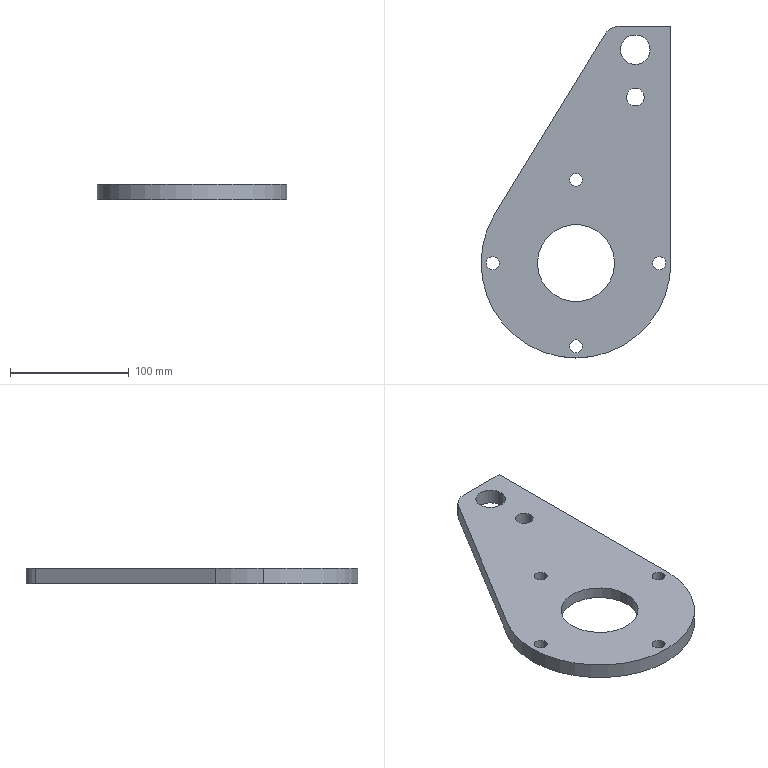Part | SolidWorks | features ICE 2, Extrusion 1 | 1 solid | 25 faces | box 160 x 280 x 13 mm | volume 339397 mm3 | cylinder 19 | plane 6 | commonest cylinder face diameters 11 x8 15 x2 25 x2 65 x2 121 x2 160 x2
STEP:
#1=CARTESIAN_POINT('',(-64.75,0.,13.));
#2=VERTEX_POINT('',#1);
#3=CARTESIAN_POINT('',(-75.75,0.,13.));
#4=VERTEX_POINT('',#3);
#5=CARTESIAN_POINT('',(-70.25,0.,13.));
#6=DIRECTION('',(0.,0.,-1.));
#7=DIRECTION('',(-1.,0.,0.));
#8=AXIS2_PLACEMENT_3D('',#5,#6,#7);
#9=CIRCLE('',#8,5.5);
#10=EDGE_CURVE('',#2,#4,#9,.T.);
#11=ORIENTED_EDGE('',*,*,#10,.F.);
#12=CARTESIAN_POINT('',(-64.75,0.,0.));
#13=VERTEX_POINT('',#12);
#14=CARTESIAN_POINT('',(-64.75,0.,13.));
#15=DIRECTION('',(0.,0.,-1.));
#16=VECTOR('',#15,1000.);
#17=LINE('',#14,#16);
#18=EDGE_CURVE('',#2,#13,#17,.T.);
#19=ORIENTED_EDGE('',*,*,#18,.T.);
#20=CARTESIAN_POINT('',(-75.75,0.,0.));
#21=VERTEX_POINT('',#20);
#22=CARTESIAN_POINT('',(-70.25,0.,0.));
#23=DIRECTION('',(0.,0.,-1.));
#24=DIRECTION('',(-1.,0.,0.));
#25=AXIS2_PLACEMENT_3D('',#22,#23,#24);
#26=CIRCLE('',#25,5.5);
#27=EDGE_CURVE('',#13,#21,#26,.T.);
#28=ORIENTED_EDGE('',*,*,#27,.T.);
#29=CARTESIAN_POINT('',(-75.75,0.,13.));
#30=DIRECTION('',(0.,0.,-1.));
#31=VECTOR('',#30,1000.);
#32=LINE('',#29,#31);
#33=EDGE_CURVE('',#4,#21,#32,.T.);
#34=ORIENTED_EDGE('',*,*,#33,.F.);
#35=EDGE_LOOP('',(#11,#19,#28,#34));
#36=FACE_OUTER_BOUND('',#35,.T.);
#37=CARTESIAN_POINT('',(-70.25,0.,13.));
#38=DIRECTION('',(0.,0.,-1.));
#39=DIRECTION('',(-1.,0.,0.));
#40=AXIS2_PLACEMENT_3D('',#37,#38,#39);
#41=CYLINDRICAL_SURFACE('',#40,5.5);
#42=ADVANCED_FACE('',(#36),#41,.F.);
#43=CARTESIAN_POINT('',(5.5,-70.25,13.));
#44=VERTEX_POINT('',#43);
#45=CARTESIAN_POINT('',(-5.5,-70.25,13.));
#46=VERTEX_POINT('',#45);
#47=CARTESIAN_POINT('',(0.,-70.25,13.));
#48=DIRECTION('',(0.,0.,-1.));
#49=DIRECTION('',(-1.,0.,0.));
#50=AXIS2_PLACEMENT_3D('',#47,#48,#49);
#51=CIRCLE('',#50,5.5);
#52=EDGE_CURVE('',#44,#46,#51,.T.);
#53=ORIENTED_EDGE('',*,*,#52,.F.);
#54=CARTESIAN_POINT('',(5.5,-70.25,0.));
#55=VERTEX_POINT('',#54);
#56=CARTESIAN_POINT('',(5.5,-70.25,13.));
#57=DIRECTION('',(0.,0.,-1.));
#58=VECTOR('',#57,1000.);
#59=LINE('',#56,#58);
#60=EDGE_CURVE('',#44,#55,#59,.T.);
#61=ORIENTED_EDGE('',*,*,#60,.T.);
#62=CARTESIAN_POINT('',(-5.5,-70.25,0.));
#63=VERTEX_POINT('',#62);
#64=CARTESIAN_POINT('',(0.,-70.25,0.));
#65=DIRECTION('',(0.,0.,-1.));
#66=DIRECTION('',(-1.,0.,0.));
#67=AXIS2_PLACEMENT_3D('',#64,#65,#66);
#68=CIRCLE('',#67,5.5);
#69=EDGE_CURVE('',#55,#63,#68,.T.);
#70=ORIENTED_EDGE('',*,*,#69,.T.);
#71=CARTESIAN_POINT('',(-5.5,-70.25,13.));
#72=DIRECTION('',(0.,0.,-1.));
#73=VECTOR('',#72,1000.);
#74=LINE('',#71,#73);
#75=EDGE_CURVE('',#46,#63,#74,.T.);
#76=ORIENTED_EDGE('',*,*,#75,.F.);
#77=EDGE_LOOP('',(#53,#61,#70,#76));
#78=FACE_OUTER_BOUND('',#77,.T.);
#79=CARTESIAN_POINT('',(0.,-70.25,13.));
#80=DIRECTION('',(0.,0.,-1.));
#81=DIRECTION('',(-1.,0.,0.));
#82=AXIS2_PLACEMENT_3D('',#79,#80,#81);
#83=CYLINDRICAL_SURFACE('',#82,5.5);
#84=ADVANCED_FACE('',(#78),#83,.F.);
#85=CARTESIAN_POINT('',(75.75,0.,13.));
#86=VERTEX_POINT('',#85);
#87=CARTESIAN_POINT('',(64.75,0.,13.));
#88=VERTEX_POINT('',#87);
#89=CARTESIAN_POINT('',(70.25,0.,13.));
#90=DIRECTION('',(0.,0.,-1.));
#91=DIRECTION('',(-1.,0.,0.));
#92=AXIS2_PLACEMENT_3D('',#89,#90,#91);
#93=CIRCLE('',#92,5.5);
#94=EDGE_CURVE('',#86,#88,#93,.T.);
#95=ORIENTED_EDGE('',*,*,#94,.F.);
#96=CARTESIAN_POINT('',(75.75,0.,0.));
#97=VERTEX_POINT('',#96);
#98=CARTESIAN_POINT('',(75.75,0.,13.));
#99=DIRECTION('',(0.,0.,-1.));
#100=VECTOR('',#99,1000.);
#101=LINE('',#98,#100);
#102=EDGE_CURVE('',#86,#97,#101,.T.);
#103=ORIENTED_EDGE('',*,*,#102,.T.);
#104=CARTESIAN_POINT('',(64.75,0.,0.));
#105=VERTEX_POINT('',#104);
#106=CARTESIAN_POINT('',(70.25,0.,0.));
#107=DIRECTION('',(0.,0.,-1.));
#108=DIRECTION('',(-1.,0.,0.));
#109=AXIS2_PLACEMENT_3D('',#106,#107,#108);
#110=CIRCLE('',#109,5.5);
#111=EDGE_CURVE('',#97,#105,#110,.T.);
#112=ORIENTED_EDGE('',*,*,#111,.T.);
#113=CARTESIAN_POINT('',(64.75,0.,13.));
#114=DIRECTION('',(0.,0.,-1.));
#115=VECTOR('',#114,1000.);
#116=LINE('',#113,#115);
#117=EDGE_CURVE('',#88,#105,#116,.T.);
#118=ORIENTED_EDGE('',*,*,#117,.F.);
#119=EDGE_LOOP('',(#95,#103,#112,#118));
#120=FACE_OUTER_BOUND('',#119,.T.);
#121=CARTESIAN_POINT('',(70.25,0.,13.));
#122=DIRECTION('',(0.,0.,-1.));
#123=DIRECTION('',(-1.,0.,0.));
#124=AXIS2_PLACEMENT_3D('',#121,#122,#123);
#125=CYLINDRICAL_SURFACE('',#124,5.5);
#126=ADVANCED_FACE('',(#120),#125,.F.);
#127=CARTESIAN_POINT('',(5.5,70.25,13.));
#128=VERTEX_POINT('',#127);
#129=CARTESIAN_POINT('',(-5.5,70.25,13.));
#130=VERTEX_POINT('',#129);
#131=CARTESIAN_POINT('',(0.,70.25,13.));
#132=DIRECTION('',(0.,0.,-1.));
#133=DIRECTION('',(-1.,0.,0.));
#134=AXIS2_PLACEMENT_3D('',#131,#132,#133);
#135=CIRCLE('',#134,5.5);
#136=EDGE_CURVE('',#128,#130,#135,.T.);
#137=ORIENTED_EDGE('',*,*,#136,.F.);
#138=CARTESIAN_POINT('',(5.5,70.25,0.));
#139=VERTEX_POINT('',#138);
#140=CARTESIAN_POINT('',(5.5,70.25,13.));
#141=DIRECTION('',(0.,0.,-1.));
#142=VECTOR('',#141,1000.);
#143=LINE('',#140,#142);
#144=EDGE_CURVE('',#128,#139,#143,.T.);
#145=ORIENTED_EDGE('',*,*,#144,.T.);
#146=CARTESIAN_POINT('',(-5.5,70.25,0.));
#147=VERTEX_POINT('',#146);
#148=CARTESIAN_POINT('',(0.,70.25,0.));
#149=DIRECTION('',(0.,0.,-1.));
#150=DIRECTION('',(-1.,0.,0.));
#151=AXIS2_PLACEMENT_3D('',#148,#149,#150);
#152=CIRCLE('',#151,5.5);
#153=EDGE_CURVE('',#139,#147,#152,.T.);
#154=ORIENTED_EDGE('',*,*,#153,.T.);
#155=CARTESIAN_POINT('',(-5.5,70.25,13.));
#156=DIRECTION('',(0.,0.,-1.));
#157=VECTOR('',#156,1000.);
#158=LINE('',#155,#157);
#159=EDGE_CURVE('',#130,#147,#158,.T.);
#160=ORIENTED_EDGE('',*,*,#159,.F.);
#161=EDGE_LOOP('',(#137,#145,#154,#160));
#162=FACE_OUTER_BOUND('',#161,.T.);
#163=CARTESIAN_POINT('',(0.,70.25,13.));
#164=DIRECTION('',(0.,0.,-1.));
#165=DIRECTION('',(-1.,0.,0.));
#166=AXIS2_PLACEMENT_3D('',#163,#164,#165);
#167=CYLINDRICAL_SURFACE('',#166,5.5);
#168=ADVANCED_FACE('',(#162),#167,.F.);
#169=CARTESIAN_POINT('',(-60.5,0.,0.));
#170=VERTEX_POINT('',#169);
#171=CARTESIAN_POINT('',(60.5,0.,0.));
#172=VERTEX_POINT('',#171);
#173=CARTESIAN_POINT('',(0.,0.,0.));
#174=DIRECTION('',(0.,0.,1.));
#175=DIRECTION('',(1.,0.,0.));
#176=AXIS2_PLACEMENT_3D('',#173,#174,#175);
#177=CIRCLE('',#176,60.5);
#178=EDGE_CURVE('',#170,#172,#177,.T.);
#179=ORIENTED_EDGE('',*,*,#178,.F.);
#180=CARTESIAN_POINT('',(-60.5,0.,3.));
#181=VERTEX_POINT('',#180);
#182=CARTESIAN_POINT('',(-60.5,0.,0.));
#183=DIRECTION('',(0.,0.,1.));
#184=VECTOR('',#183,1000.);
#185=LINE('',#182,#184);
#186=EDGE_CURVE('',#170,#181,#185,.T.);
#187=ORIENTED_EDGE('',*,*,#186,.T.);
#188=CARTESIAN_POINT('',(60.5,0.,3.));
#189=VERTEX_POINT('',#188);
#190=CARTESIAN_POINT('',(0.,0.,3.));
#191=DIRECTION('',(0.,0.,1.));
#192=DIRECTION('',(1.,0.,0.));
#193=AXIS2_PLACEMENT_3D('',#190,#191,#192);
#194=CIRCLE('',#193,60.5);
#195=EDGE_CURVE('',#181,#189,#194,.T.);
#196=ORIENTED_EDGE('',*,*,#195,.T.);
#197=CARTESIAN_POINT('',(60.5,0.,0.));
#198=DIRECTION('',(0.,0.,1.));
#199=VECTOR('',#198,1000.);
#200=LINE('',#197,#199);
#201=EDGE_CURVE('',#172,#189,#200,.T.);
#202=ORIENTED_EDGE('',*,*,#201,.F.);
#203=EDGE_LOOP('',(#179,#187,#196,#202));
#204=FACE_OUTER_BOUND('',#203,.T.);
#205=CARTESIAN_POINT('',(0.,0.,0.));
#206=DIRECTION('',(0.,0.,1.));
#207=DIRECTION('',(1.,0.,0.));
#208=AXIS2_PLACEMENT_3D('',#205,#206,#207);
#209=CYLINDRICAL_SURFACE('',#208,60.5);
#210=ADVANCED_FACE('',(#204),#209,.F.);
#211=CARTESIAN_POINT('',(42.5,140.,13.));
#212=VERTEX_POINT('',#211);
#213=CARTESIAN_POINT('',(57.5,140.,13.));
#214=VERTEX_POINT('',#213);
#215=CARTESIAN_POINT('',(50.,140.,13.));
#216=DIRECTION('',(0.,0.,1.));
#217=DIRECTION('',(1.,0.,0.));
#218=AXIS2_PLACEMENT_3D('',#215,#216,#217);
#219=CIRCLE('',#218,7.5);
#220=EDGE_CURVE('',#212,#214,#219,.T.);
#221=ORIENTED_EDGE('',*,*,#220,.T.);
#222=CARTESIAN_POINT('',(57.5,140.,0.));
#223=VERTEX_POINT('',#222);
#224=CARTESIAN_POINT('',(57.5,140.,13.));
#225=DIRECTION('',(0.,0.,-1.));
#226=VECTOR('',#225,1000.);
#227=LINE('',#224,#226);
#228=EDGE_CURVE('',#214,#223,#227,.T.);
#229=ORIENTED_EDGE('',*,*,#228,.T.);
#230=CARTESIAN_POINT('',(42.5,140.,0.));
#231=VERTEX_POINT('',#230);
#232=CARTESIAN_POINT('',(50.,140.,0.));
#233=DIRECTION('',(0.,0.,1.));
#234=DIRECTION('',(1.,0.,0.));
#235=AXIS2_PLACEMENT_3D('',#232,#233,#234);
#236=CIRCLE('',#235,7.5);
#237=EDGE_CURVE('',#231,#223,#236,.T.);
#238=ORIENTED_EDGE('',*,*,#237,.F.);
#239=CARTESIAN_POINT('',(42.5,140.,13.));
#240=DIRECTION('',(0.,0.,-1.));
#241=VECTOR('',#240,1000.);
#242=LINE('',#239,#241);
#243=EDGE_CURVE('',#212,#231,#242,.T.);
#244=ORIENTED_EDGE('',*,*,#243,.F.);
#245=EDGE_LOOP('',(#221,#229,#238,#244));
#246=FACE_OUTER_BOUND('',#245,.T.);
#247=CARTESIAN_POINT('',(50.,140.,13.));
#248=DIRECTION('',(0.,0.,-1.));
#249=DIRECTION('',(-1.,0.,0.));
#250=AXIS2_PLACEMENT_3D('',#247,#248,#249);
#251=CYLINDRICAL_SURFACE('',#250,7.5);
#252=ADVANCED_FACE('',(#246),#251,.F.);
#253=CARTESIAN_POINT('',(-32.5,0.,13.));
#254=VERTEX_POINT('',#253);
#255=CARTESIAN_POINT('',(32.5,0.,13.));
#256=VERTEX_POINT('',#255);
#257=CARTESIAN_POINT('',(0.,0.,13.));
#258=DIRECTION('',(0.,0.,1.));
#259=DIRECTION('',(1.,0.,0.));
#260=AXIS2_PLACEMENT_3D('',#257,#258,#259);
#261=CIRCLE('',#260,32.5);
#262=EDGE_CURVE('',#254,#256,#261,.T.);
#263=ORIENTED_EDGE('',*,*,#262,.T.);
#264=CARTESIAN_POINT('',(32.5,0.,3.));
#265=VERTEX_POINT('',#264);
#266=CARTESIAN_POINT('',(32.5,0.,13.));
#267=DIRECTION('',(0.,0.,-1.));
#268=VECTOR('',#267,1000.);
#269=LINE('',#266,#268);
#270=EDGE_CURVE('',#256,#265,#269,.T.);
#271=ORIENTED_EDGE('',*,*,#270,.T.);
#272=CARTESIAN_POINT('',(-32.5,0.,3.));
#273=VERTEX_POINT('',#272);
#274=CARTESIAN_POINT('',(0.,0.,3.));
#275=DIRECTION('',(0.,0.,1.));
#276=DIRECTION('',(1.,0.,0.));
#277=AXIS2_PLACEMENT_3D('',#274,#275,#276);
#278=CIRCLE('',#277,32.5);
#279=EDGE_CURVE('',#273,#265,#278,.T.);
#280=ORIENTED_EDGE('',*,*,#279,.F.);
#281=CARTESIAN_POINT('',(-32.5,0.,13.));
#282=DIRECTION('',(0.,0.,-1.));
#283=VECTOR('',#282,1000.);
#284=LINE('',#281,#283);
#285=EDGE_CURVE('',#254,#273,#284,.T.);
#286=ORIENTED_EDGE('',*,*,#285,.F.);
#287=EDGE_LOOP('',(#263,#271,#280,#286));
#288=FACE_OUTER_BOUND('',#287,.T.);
#289=CARTESIAN_POINT('',(0.,0.,13.));
#290=DIRECTION('',(0.,0.,-1.));
#291=DIRECTION('',(-1.,0.,0.));
#292=AXIS2_PLACEMENT_3D('',#289,#290,#291);
#293=CYLINDRICAL_SURFACE('',#292,32.5);
#294=ADVANCED_FACE('',(#288),#293,.F.);
#295=CARTESIAN_POINT('',(37.5,180.,13.));
#296=VERTEX_POINT('',#295);
#297=CARTESIAN_POINT('',(62.5,180.,13.));
#298=VERTEX_POINT('',#297);
#299=CARTESIAN_POINT('',(50.,180.,13.));
#300=DIRECTION('',(0.,0.,1.));
#301=DIRECTION('',(1.,0.,0.));
#302=AXIS2_PLACEMENT_3D('',#299,#300,#301);
#303=CIRCLE('',#302,12.5);
#304=EDGE_CURVE('',#296,#298,#303,.T.);
#305=ORIENTED_EDGE('',*,*,#304,.T.);
#306=CARTESIAN_POINT('',(62.5,180.,0.));
#307=VERTEX_POINT('',#306);
#308=CARTESIAN_POINT('',(62.5,180.,13.));
#309=DIRECTION('',(0.,0.,-1.));
#310=VECTOR('',#309,1000.);
#311=LINE('',#308,#310);
#312=EDGE_CURVE('',#298,#307,#311,.T.);
#313=ORIENTED_EDGE('',*,*,#312,.T.);
#314=CARTESIAN_POINT('',(37.5,180.,0.));
#315=VERTEX_POINT('',#314);
#316=CARTESIAN_POINT('',(50.,180.,0.));
#317=DIRECTION('',(0.,0.,1.));
#318=DIRECTION('',(1.,0.,0.));
#319=AXIS2_PLACEMENT_3D('',#316,#317,#318);
#320=CIRCLE('',#319,12.5);
#321=EDGE_CURVE('',#315,#307,#320,.T.);
#322=ORIENTED_EDGE('',*,*,#321,.F.);
#323=CARTESIAN_POINT('',(37.5,180.,13.));
#324=DIRECTION('',(0.,0.,-1.));
#325=VECTOR('',#324,1000.);
#326=LINE('',#323,#325);
#327=EDGE_CURVE('',#296,#315,#326,.T.);
#328=ORIENTED_EDGE('',*,*,#327,.F.);
#329=EDGE_LOOP('',(#305,#313,#322,#328));
#330=FACE_OUTER_BOUND('',#329,.T.);
#331=CARTESIAN_POINT('',(50.,180.,13.));
#332=DIRECTION('',(0.,0.,-1.));
#333=DIRECTION('',(-1.,0.,0.));
#334=AXIS2_PLACEMENT_3D('',#331,#332,#333);
#335=CYLINDRICAL_SURFACE('',#334,12.5);
#336=ADVANCED_FACE('',(#330),#335,.F.);
#337=CARTESIAN_POINT('',(-80.,0.,13.));
#338=VERTEX_POINT('',#337);
#339=CARTESIAN_POINT('',(80.,0.,13.));
#340=VERTEX_POINT('',#339);
#341=CARTESIAN_POINT('',(0.,0.,13.));
#342=DIRECTION('',(0.,0.,1.));
#343=DIRECTION('',(1.,0.,0.));
#344=AXIS2_PLACEMENT_3D('',#341,#342,#343);
#345=CIRCLE('',#344,80.);
#346=EDGE_CURVE('',#338,#340,#345,.T.);
#347=ORIENTED_EDGE('',*,*,#346,.F.);
#348=CARTESIAN_POINT('',(-80.,0.,0.));
#349=VERTEX_POINT('',#348);
#350=CARTESIAN_POINT('',(-80.,0.,13.));
#351=DIRECTION('',(0.,0.,-1.));
#352=VECTOR('',#351,1000.);
#353=LINE('',#350,#352);
#354=EDGE_CURVE('',#338,#349,#353,.T.);
#355=ORIENTED_EDGE('',*,*,#354,.T.);
#356=CARTESIAN_POINT('',(80.,0.,0.));
#357=VERTEX_POINT('',#356);
#358=CARTESIAN_POINT('',(0.,0.,0.));
#359=DIRECTION('',(0.,0.,1.));
#360=DIRECTION('',(1.,0.,0.));
#361=AXIS2_PLACEMENT_3D('',#358,#359,#360);
#362=CIRCLE('',#361,80.);
#363=EDGE_CURVE('',#349,#357,#362,.T.);
#364=ORIENTED_EDGE('',*,*,#363,.T.);
#365=CARTESIAN_POINT('',(80.,0.,13.));
#366=DIRECTION('',(0.,0.,-1.));
#367=VECTOR('',#366,1000.);
#368=LINE('',#365,#367);
#369=EDGE_CURVE('',#340,#357,#368,.T.);
#370=ORIENTED_EDGE('',*,*,#369,.F.);
#371=EDGE_LOOP('',(#347,#355,#364,#370));
#372=FACE_OUTER_BOUND('',#371,.T.);
#373=CARTESIAN_POINT('',(0.,0.,13.));
#374=DIRECTION('',(0.,0.,-1.));
#375=DIRECTION('',(-1.,0.,0.));
#376=AXIS2_PLACEMENT_3D('',#373,#374,#375);
#377=CYLINDRICAL_SURFACE('',#376,80.);
#378=ADVANCED_FACE('',(#372),#377,.T.);
#379=CARTESIAN_POINT('',(-70.25,0.,13.));
#380=DIRECTION('',(0.,0.,-1.));
#381=DIRECTION('',(-1.,0.,0.));
#382=AXIS2_PLACEMENT_3D('',#379,#380,#381);
#383=CIRCLE('',#382,5.5);
#384=EDGE_CURVE('',#4,#2,#383,.T.);
#385=ORIENTED_EDGE('',*,*,#384,.T.);
#386=ORIENTED_EDGE('',*,*,#10,.T.);
#387=EDGE_LOOP('',(#385,#386));
#388=FACE_BOUND('',#387,.T.);
#389=CARTESIAN_POINT('',(0.,-70.25,13.));
#390=DIRECTION('',(0.,0.,-1.));
#391=DIRECTION('',(-1.,0.,0.));
#392=AXIS2_PLACEMENT_3D('',#389,#390,#391);
#393=CIRCLE('',#392,5.5);
#394=EDGE_CURVE('',#46,#44,#393,.T.);
#395=ORIENTED_EDGE('',*,*,#394,.T.);
#396=ORIENTED_EDGE('',*,*,#52,.T.);
#397=EDGE_LOOP('',(#395,#396));
#398=FACE_BOUND('',#397,.T.);
#399=CARTESIAN_POINT('',(70.25,0.,13.));
#400=DIRECTION('',(0.,0.,-1.));
#401=DIRECTION('',(-1.,0.,0.));
#402=AXIS2_PLACEMENT_3D('',#399,#400,#401);
#403=CIRCLE('',#402,5.5);
#404=EDGE_CURVE('',#88,#86,#403,.T.);
#405=ORIENTED_EDGE('',*,*,#404,.T.);
#406=ORIENTED_EDGE('',*,*,#94,.T.);
#407=EDGE_LOOP('',(#405,#406));
#408=FACE_BOUND('',#407,.T.);
#409=CARTESIAN_POINT('',(0.,70.25,13.));
#410=DIRECTION('',(0.,0.,-1.));
#411=DIRECTION('',(-1.,0.,0.));
#412=AXIS2_PLACEMENT_3D('',#409,#410,#411);
#413=CIRCLE('',#412,5.5);
#414=EDGE_CURVE('',#130,#128,#413,.T.);
#415=ORIENTED_EDGE('',*,*,#414,.T.);
#416=ORIENTED_EDGE('',*,*,#136,.T.);
#417=EDGE_LOOP('',(#415,#416));
#418=FACE_BOUND('',#417,.T.);
#419=ORIENTED_EDGE('',*,*,#262,.F.);
#420=CARTESIAN_POINT('',(0.,0.,13.));
#421=DIRECTION('',(0.,0.,1.));
#422=DIRECTION('',(1.,0.,0.));
#423=AXIS2_PLACEMENT_3D('',#420,#421,#422);
#424=CIRCLE('',#423,32.5);
#425=EDGE_CURVE('',#256,#254,#424,.T.);
#426=ORIENTED_EDGE('',*,*,#425,.F.);
#427=EDGE_LOOP('',(#419,#426));
#428=FACE_BOUND('',#427,.T.);
#429=CARTESIAN_POINT('',(-69.389,39.815,13.));
#430=VERTEX_POINT('',#429);
#431=CARTESIAN_POINT('',(0.,0.,13.));
#432=DIRECTION('',(0.,0.,1.));
#433=DIRECTION('',(1.,0.,0.));
#434=AXIS2_PLACEMENT_3D('',#431,#432,#433);
#435=CIRCLE('',#434,80.);
#436=EDGE_CURVE('',#430,#338,#435,.T.);
#437=ORIENTED_EDGE('',*,*,#436,.T.);
#438=ORIENTED_EDGE('',*,*,#346,.T.);
#439=CARTESIAN_POINT('',(80.,200.,13.));
#440=VERTEX_POINT('',#439);
#441=CARTESIAN_POINT('',(80.,0.,13.));
#442=DIRECTION('',(0.,1.,0.));
#443=VECTOR('',#442,1000.);
#444=LINE('',#441,#443);
#445=EDGE_CURVE('',#340,#440,#444,.T.);
#446=ORIENTED_EDGE('',*,*,#445,.T.);
#447=CARTESIAN_POINT('',(37.5,200.,13.));
#448=VERTEX_POINT('',#447);
#449=CARTESIAN_POINT('',(80.,200.,13.));
#450=DIRECTION('',(-1.,0.,0.));
#451=VECTOR('',#450,1000.);
#452=LINE('',#449,#451);
#453=EDGE_CURVE('',#440,#448,#452,.T.);
#454=ORIENTED_EDGE('',*,*,#453,.T.);
#455=CARTESIAN_POINT('',(23.848,192.345,13.));
#456=VERTEX_POINT('',#455);
#457=CARTESIAN_POINT('',(37.5,184.,13.));
#458=DIRECTION('',(0.,0.,1.));
#459=DIRECTION('',(1.,0.,0.));
#460=AXIS2_PLACEMENT_3D('',#457,#458,#459);
#461=CIRCLE('',#460,16.);
#462=EDGE_CURVE('',#448,#456,#461,.T.);
#463=ORIENTED_EDGE('',*,*,#462,.T.);
#464=CARTESIAN_POINT('',(-69.389,39.815,13.));
#465=DIRECTION('',(-0.5215,-0.8532,0.));
#466=VECTOR('',#465,1000.);
#467=LINE('',#464,#466);
#468=EDGE_CURVE('',#456,#430,#467,.T.);
#469=ORIENTED_EDGE('',*,*,#468,.T.);
#470=EDGE_LOOP('',(#437,#438,#446,#454,#463,#469));
#471=FACE_OUTER_BOUND('',#470,.T.);
#472=ORIENTED_EDGE('',*,*,#304,.F.);
#473=CARTESIAN_POINT('',(50.,180.,13.));
#474=DIRECTION('',(0.,0.,1.));
#475=DIRECTION('',(1.,0.,0.));
#476=AXIS2_PLACEMENT_3D('',#473,#474,#475);
#477=CIRCLE('',#476,12.5);
#478=EDGE_CURVE('',#298,#296,#477,.T.);
#479=ORIENTED_EDGE('',*,*,#478,.F.);
#480=EDGE_LOOP('',(#472,#479));
#481=FACE_BOUND('',#480,.T.);
#482=ORIENTED_EDGE('',*,*,#220,.F.);
#483=CARTESIAN_POINT('',(50.,140.,13.));
#484=DIRECTION('',(0.,0.,1.));
#485=DIRECTION('',(1.,0.,0.));
#486=AXIS2_PLACEMENT_3D('',#483,#484,#485);
#487=CIRCLE('',#486,7.5);
#488=EDGE_CURVE('',#214,#212,#487,.T.);
#489=ORIENTED_EDGE('',*,*,#488,.F.);
#490=EDGE_LOOP('',(#482,#489));
#491=FACE_BOUND('',#490,.T.);
#492=CARTESIAN_POINT('',(0.,0.,13.));
#493=DIRECTION('',(0.,0.,1.));
#494=DIRECTION('',(1.,0.,0.));
#495=AXIS2_PLACEMENT_3D('',#492,#493,#494);
#496=PLANE('',#495);
#497=ADVANCED_FACE('',(#388,#398,#408,#418,#428,#471,#481,#491),#496,.T.);
#498=CARTESIAN_POINT('',(-70.25,0.,0.));
#499=DIRECTION('',(0.,0.,-1.));
#500=DIRECTION('',(-1.,0.,0.));
#501=AXIS2_PLACEMENT_3D('',#498,#499,#500);
#502=CIRCLE('',#501,5.5);
#503=EDGE_CURVE('',#21,#13,#502,.T.);
#504=ORIENTED_EDGE('',*,*,#503,.F.);
#505=ORIENTED_EDGE('',*,*,#27,.F.);
#506=EDGE_LOOP('',(#504,#505));
#507=FACE_BOUND('',#506,.T.);
#508=CARTESIAN_POINT('',(0.,-70.25,0.));
#509=DIRECTION('',(0.,0.,-1.));
#510=DIRECTION('',(-1.,0.,0.));
#511=AXIS2_PLACEMENT_3D('',#508,#509,#510);
#512=CIRCLE('',#511,5.5);
#513=EDGE_CURVE('',#63,#55,#512,.T.);
#514=ORIENTED_EDGE('',*,*,#513,.F.);
#515=ORIENTED_EDGE('',*,*,#69,.F.);
#516=EDGE_LOOP('',(#514,#515));
#517=FACE_BOUND('',#516,.T.);
#518=CARTESIAN_POINT('',(70.25,0.,0.));
#519=DIRECTION('',(0.,0.,-1.));
#520=DIRECTION('',(-1.,0.,0.));
#521=AXIS2_PLACEMENT_3D('',#518,#519,#520);
#522=CIRCLE('',#521,5.5);
#523=EDGE_CURVE('',#105,#97,#522,.T.);
#524=ORIENTED_EDGE('',*,*,#523,.F.);
#525=ORIENTED_EDGE('',*,*,#111,.F.);
#526=EDGE_LOOP('',(#524,#525));
#527=FACE_BOUND('',#526,.T.);
#528=CARTESIAN_POINT('',(0.,70.25,0.));
#529=DIRECTION('',(0.,0.,-1.));
#530=DIRECTION('',(-1.,0.,0.));
#531=AXIS2_PLACEMENT_3D('',#528,#529,#530);
#532=CIRCLE('',#531,5.5);
#533=EDGE_CURVE('',#147,#139,#532,.T.);
#534=ORIENTED_EDGE('',*,*,#533,.F.);
#535=ORIENTED_EDGE('',*,*,#153,.F.);
#536=EDGE_LOOP('',(#534,#535));
#537=FACE_BOUND('',#536,.T.);
#538=CARTESIAN_POINT('',(0.,0.,0.));
#539=DIRECTION('',(0.,0.,1.));
#540=DIRECTION('',(1.,0.,0.));
#541=AXIS2_PLACEMENT_3D('',#538,#539,#540);
#542=CIRCLE('',#541,60.5);
#543=EDGE_CURVE('',#172,#170,#542,.T.);
#544=ORIENTED_EDGE('',*,*,#543,.T.);
#545=ORIENTED_EDGE('',*,*,#178,.T.);
#546=EDGE_LOOP('',(#544,#545));
#547=FACE_BOUND('',#546,.T.);
#548=CARTESIAN_POINT('',(-69.389,39.815,0.));
#549=VERTEX_POINT('',#548);
#550=CARTESIAN_POINT('',(0.,0.,0.));
#551=DIRECTION('',(0.,0.,1.));
#552=DIRECTION('',(1.,0.,0.));
#553=AXIS2_PLACEMENT_3D('',#550,#551,#552);
#554=CIRCLE('',#553,80.);
#555=EDGE_CURVE('',#549,#349,#554,.T.);
#556=ORIENTED_EDGE('',*,*,#555,.F.);
#557=CARTESIAN_POINT('',(23.848,192.345,0.));
#558=VERTEX_POINT('',#557);
#559=CARTESIAN_POINT('',(-69.389,39.815,0.));
#560=DIRECTION('',(-0.5215,-0.8532,0.));
#561=VECTOR('',#560,1000.);
#562=LINE('',#559,#561);
#563=EDGE_CURVE('',#558,#549,#562,.T.);
#564=ORIENTED_EDGE('',*,*,#563,.F.);
#565=CARTESIAN_POINT('',(37.5,200.,0.));
#566=VERTEX_POINT('',#565);
#567=CARTESIAN_POINT('',(37.5,184.,0.));
#568=DIRECTION('',(0.,0.,1.));
#569=DIRECTION('',(1.,0.,0.));
#570=AXIS2_PLACEMENT_3D('',#567,#568,#569);
#571=CIRCLE('',#570,16.);
#572=EDGE_CURVE('',#566,#558,#571,.T.);
#573=ORIENTED_EDGE('',*,*,#572,.F.);
#574=CARTESIAN_POINT('',(80.,200.,0.));
#575=VERTEX_POINT('',#574);
#576=CARTESIAN_POINT('',(80.,200.,0.));
#577=DIRECTION('',(-1.,0.,0.));
#578=VECTOR('',#577,1000.);
#579=LINE('',#576,#578);
#580=EDGE_CURVE('',#575,#566,#579,.T.);
#581=ORIENTED_EDGE('',*,*,#580,.F.);
#582=CARTESIAN_POINT('',(80.,200.,0.));
#583=DIRECTION('',(0.,1.,0.));
#584=VECTOR('',#583,1000.);
#585=LINE('',#582,#584);
#586=EDGE_CURVE('',#357,#575,#585,.T.);
#587=ORIENTED_EDGE('',*,*,#586,.F.);
#588=ORIENTED_EDGE('',*,*,#363,.F.);
#589=EDGE_LOOP('',(#556,#564,#573,#581,#587,#588));
#590=FACE_OUTER_BOUND('',#589,.T.);
#591=ORIENTED_EDGE('',*,*,#321,.T.);
#592=CARTESIAN_POINT('',(50.,180.,0.));
#593=DIRECTION('',(0.,0.,1.));
#594=DIRECTION('',(1.,0.,0.));
#595=AXIS2_PLACEMENT_3D('',#592,#593,#594);
#596=CIRCLE('',#595,12.5);
#597=EDGE_CURVE('',#307,#315,#596,.T.);
#598=ORIENTED_EDGE('',*,*,#597,.T.);
#599=EDGE_LOOP('',(#591,#598));
#600=FACE_BOUND('',#599,.T.);
#601=ORIENTED_EDGE('',*,*,#237,.T.);
#602=CARTESIAN_POINT('',(50.,140.,0.));
#603=DIRECTION('',(0.,0.,1.));
#604=DIRECTION('',(1.,0.,0.));
#605=AXIS2_PLACEMENT_3D('',#602,#603,#604);
#606=CIRCLE('',#605,7.5);
#607=EDGE_CURVE('',#223,#231,#606,.T.);
#608=ORIENTED_EDGE('',*,*,#607,.T.);
#609=EDGE_LOOP('',(#601,#608));
#610=FACE_BOUND('',#609,.T.);
#611=CARTESIAN_POINT('',(0.,0.,0.));
#612=DIRECTION('',(0.,0.,1.));
#613=DIRECTION('',(1.,0.,0.));
#614=AXIS2_PLACEMENT_3D('',#611,#612,#613);
#615=PLANE('',#614);
#616=ADVANCED_FACE('',(#507,#517,#527,#537,#547,#590,#600,#610),#615,.F.);
#617=ORIENTED_EDGE('',*,*,#354,.F.);
#618=ORIENTED_EDGE('',*,*,#436,.F.);
#619=CARTESIAN_POINT('',(-69.389,39.815,13.));
#620=DIRECTION('',(0.,0.,-1.));
#621=VECTOR('',#620,1000.);
#622=LINE('',#619,#621);
#623=EDGE_CURVE('',#430,#549,#622,.T.);
#624=ORIENTED_EDGE('',*,*,#623,.T.);
#625=ORIENTED_EDGE('',*,*,#555,.T.);
#626=EDGE_LOOP('',(#617,#618,#624,#625));
#627=FACE_OUTER_BOUND('',#626,.T.);
#628=CARTESIAN_POINT('',(0.,0.,13.));
#629=DIRECTION('',(0.,0.,-1.));
#630=DIRECTION('',(-1.,0.,0.));
#631=AXIS2_PLACEMENT_3D('',#628,#629,#630);
#632=CYLINDRICAL_SURFACE('',#631,80.);
#633=ADVANCED_FACE('',(#627),#632,.T.);
#634=ORIENTED_EDGE('',*,*,#586,.T.);
#635=CARTESIAN_POINT('',(80.,200.,13.));
#636=DIRECTION('',(0.,0.,-1.));
#637=VECTOR('',#636,1000.);
#638=LINE('',#635,#637);
#639=EDGE_CURVE('',#440,#575,#638,.T.);
#640=ORIENTED_EDGE('',*,*,#639,.F.);
#641=ORIENTED_EDGE('',*,*,#445,.F.);
#642=ORIENTED_EDGE('',*,*,#369,.T.);
#643=EDGE_LOOP('',(#634,#640,#641,#642));
#644=FACE_OUTER_BOUND('',#643,.T.);
#645=CARTESIAN_POINT('',(80.,200.,13.));
#646=DIRECTION('',(-1.,0.,0.));
#647=DIRECTION('',(0.,0.,1.));
#648=AXIS2_PLACEMENT_3D('',#645,#646,#647);
#649=PLANE('',#648);
#650=ADVANCED_FACE('',(#644),#649,.F.);
#651=ORIENTED_EDGE('',*,*,#580,.T.);
#652=CARTESIAN_POINT('',(37.5,200.,13.));
#653=DIRECTION('',(0.,0.,-1.));
#654=VECTOR('',#653,1000.);
#655=LINE('',#652,#654);
#656=EDGE_CURVE('',#448,#566,#655,.T.);
#657=ORIENTED_EDGE('',*,*,#656,.F.);
#658=ORIENTED_EDGE('',*,*,#453,.F.);
#659=ORIENTED_EDGE('',*,*,#639,.T.);
#660=EDGE_LOOP('',(#651,#657,#658,#659));
#661=FACE_OUTER_BOUND('',#660,.T.);
#662=CARTESIAN_POINT('',(80.,200.,13.));
#663=DIRECTION('',(0.,-1.,0.));
#664=DIRECTION('',(0.,0.,-1.));
#665=AXIS2_PLACEMENT_3D('',#662,#663,#664);
#666=PLANE('',#665);
#667=ADVANCED_FACE('',(#661),#666,.F.);
#668=ORIENTED_EDGE('',*,*,#572,.T.);
#669=CARTESIAN_POINT('',(23.848,192.345,13.));
#670=DIRECTION('',(0.,0.,-1.));
#671=VECTOR('',#670,1000.);
#672=LINE('',#669,#671);
#673=EDGE_CURVE('',#456,#558,#672,.T.);
#674=ORIENTED_EDGE('',*,*,#673,.F.);
#675=ORIENTED_EDGE('',*,*,#462,.F.);
#676=ORIENTED_EDGE('',*,*,#656,.T.);
#677=EDGE_LOOP('',(#668,#674,#675,#676));
#678=FACE_OUTER_BOUND('',#677,.T.);
#679=CARTESIAN_POINT('',(37.5,184.,13.));
#680=DIRECTION('',(0.,0.,-1.));
#681=DIRECTION('',(-1.,0.,0.));
#682=AXIS2_PLACEMENT_3D('',#679,#680,#681);
#683=CYLINDRICAL_SURFACE('',#682,16.);
#684=ADVANCED_FACE('',(#678),#683,.T.);
#685=ORIENTED_EDGE('',*,*,#563,.T.);
#686=ORIENTED_EDGE('',*,*,#623,.F.);
#687=ORIENTED_EDGE('',*,*,#468,.F.);
#688=ORIENTED_EDGE('',*,*,#673,.T.);
#689=EDGE_LOOP('',(#685,#686,#687,#688));
#690=FACE_OUTER_BOUND('',#689,.T.);
#691=CARTESIAN_POINT('',(-69.389,39.815,13.));
#692=DIRECTION('',(0.8532,-0.5215,0.));
#693=DIRECTION('',(0.5215,0.8532,0.));
#694=AXIS2_PLACEMENT_3D('',#691,#692,#693);
#695=PLANE('',#694);
#696=ADVANCED_FACE('',(#690),#695,.F.);
#697=ORIENTED_EDGE('',*,*,#312,.F.);
#698=ORIENTED_EDGE('',*,*,#478,.T.);
#699=ORIENTED_EDGE('',*,*,#327,.T.);
#700=ORIENTED_EDGE('',*,*,#597,.F.);
#701=EDGE_LOOP('',(#697,#698,#699,#700));
#702=FACE_OUTER_BOUND('',#701,.T.);
#703=CARTESIAN_POINT('',(50.,180.,13.));
#704=DIRECTION('',(0.,0.,-1.));
#705=DIRECTION('',(-1.,0.,0.));
#706=AXIS2_PLACEMENT_3D('',#703,#704,#705);
#707=CYLINDRICAL_SURFACE('',#706,12.5);
#708=ADVANCED_FACE('',(#702),#707,.F.);
#709=ORIENTED_EDGE('',*,*,#270,.F.);
#710=ORIENTED_EDGE('',*,*,#425,.T.);
#711=ORIENTED_EDGE('',*,*,#285,.T.);
#712=CARTESIAN_POINT('',(0.,0.,3.));
#713=DIRECTION('',(0.,0.,1.));
#714=DIRECTION('',(1.,0.,0.));
#715=AXIS2_PLACEMENT_3D('',#712,#713,#714);
#716=CIRCLE('',#715,32.5);
#717=EDGE_CURVE('',#265,#273,#716,.T.);
#718=ORIENTED_EDGE('',*,*,#717,.F.);
#719=EDGE_LOOP('',(#709,#710,#711,#718));
#720=FACE_OUTER_BOUND('',#719,.T.);
#721=CARTESIAN_POINT('',(0.,0.,13.));
#722=DIRECTION('',(0.,0.,-1.));
#723=DIRECTION('',(-1.,0.,0.));
#724=AXIS2_PLACEMENT_3D('',#721,#722,#723);
#725=CYLINDRICAL_SURFACE('',#724,32.5);
#726=ADVANCED_FACE('',(#720),#725,.F.);
#727=ORIENTED_EDGE('',*,*,#228,.F.);
#728=ORIENTED_EDGE('',*,*,#488,.T.);
#729=ORIENTED_EDGE('',*,*,#243,.T.);
#730=ORIENTED_EDGE('',*,*,#607,.F.);
#731=EDGE_LOOP('',(#727,#728,#729,#730));
#732=FACE_OUTER_BOUND('',#731,.T.);
#733=CARTESIAN_POINT('',(50.,140.,13.));
#734=DIRECTION('',(0.,0.,-1.));
#735=DIRECTION('',(-1.,0.,0.));
#736=AXIS2_PLACEMENT_3D('',#733,#734,#735);
#737=CYLINDRICAL_SURFACE('',#736,7.5);
#738=ADVANCED_FACE('',(#732),#737,.F.);
#739=ORIENTED_EDGE('',*,*,#186,.F.);
#740=ORIENTED_EDGE('',*,*,#543,.F.);
#741=ORIENTED_EDGE('',*,*,#201,.T.);
#742=CARTESIAN_POINT('',(0.,0.,3.));
#743=DIRECTION('',(0.,0.,1.));
#744=DIRECTION('',(1.,0.,0.));
#745=AXIS2_PLACEMENT_3D('',#742,#743,#744);
#746=CIRCLE('',#745,60.5);
#747=EDGE_CURVE('',#189,#181,#746,.T.);
#748=ORIENTED_EDGE('',*,*,#747,.T.);
#749=EDGE_LOOP('',(#739,#740,#741,#748));
#750=FACE_OUTER_BOUND('',#749,.T.);
#751=CARTESIAN_POINT('',(0.,0.,0.));
#752=DIRECTION('',(0.,0.,1.));
#753=DIRECTION('',(1.,0.,0.));
#754=AXIS2_PLACEMENT_3D('',#751,#752,#753);
#755=CYLINDRICAL_SURFACE('',#754,60.5);
#756=ADVANCED_FACE('',(#750),#755,.F.);
#757=ORIENTED_EDGE('',*,*,#279,.T.);
#758=ORIENTED_EDGE('',*,*,#717,.T.);
#759=EDGE_LOOP('',(#757,#758));
#760=FACE_BOUND('',#759,.T.);
#761=ORIENTED_EDGE('',*,*,#747,.F.);
#762=ORIENTED_EDGE('',*,*,#195,.F.);
#763=EDGE_LOOP('',(#761,#762));
#764=FACE_OUTER_BOUND('',#763,.T.);
#765=CARTESIAN_POINT('',(0.,0.,3.));
#766=DIRECTION('',(0.,0.,1.));
#767=DIRECTION('',(1.,0.,0.));
#768=AXIS2_PLACEMENT_3D('',#765,#766,#767);
#769=PLANE('',#768);
#770=ADVANCED_FACE('',(#760,#764),#769,.F.);
#771=ORIENTED_EDGE('',*,*,#144,.F.);
#772=ORIENTED_EDGE('',*,*,#414,.F.);
#773=ORIENTED_EDGE('',*,*,#159,.T.);
#774=ORIENTED_EDGE('',*,*,#533,.T.);
#775=EDGE_LOOP('',(#771,#772,#773,#774));
#776=FACE_OUTER_BOUND('',#775,.T.);
#777=CARTESIAN_POINT('',(0.,70.25,13.));
#778=DIRECTION('',(0.,0.,-1.));
#779=DIRECTION('',(-1.,0.,0.));
#780=AXIS2_PLACEMENT_3D('',#777,#778,#779);
#781=CYLINDRICAL_SURFACE('',#780,5.5);
#782=ADVANCED_FACE('',(#776),#781,.F.);
#783=ORIENTED_EDGE('',*,*,#102,.F.);
#784=ORIENTED_EDGE('',*,*,#404,.F.);
#785=ORIENTED_EDGE('',*,*,#117,.T.);
#786=ORIENTED_EDGE('',*,*,#523,.T.);
#787=EDGE_LOOP('',(#783,#784,#785,#786));
#788=FACE_OUTER_BOUND('',#787,.T.);
#789=CARTESIAN_POINT('',(70.25,0.,13.));
#790=DIRECTION('',(0.,0.,-1.));
#791=DIRECTION('',(-1.,0.,0.));
#792=AXIS2_PLACEMENT_3D('',#789,#790,#791);
#793=CYLINDRICAL_SURFACE('',#792,5.5);
#794=ADVANCED_FACE('',(#788),#793,.F.);
#795=ORIENTED_EDGE('',*,*,#60,.F.);
#796=ORIENTED_EDGE('',*,*,#394,.F.);
#797=ORIENTED_EDGE('',*,*,#75,.T.);
#798=ORIENTED_EDGE('',*,*,#513,.T.);
#799=EDGE_LOOP('',(#795,#796,#797,#798));
#800=FACE_OUTER_BOUND('',#799,.T.);
#801=CARTESIAN_POINT('',(0.,-70.25,13.));
#802=DIRECTION('',(0.,0.,-1.));
#803=DIRECTION('',(-1.,0.,0.));
#804=AXIS2_PLACEMENT_3D('',#801,#802,#803);
#805=CYLINDRICAL_SURFACE('',#804,5.5);
#806=ADVANCED_FACE('',(#800),#805,.F.);
#807=ORIENTED_EDGE('',*,*,#18,.F.);
#808=ORIENTED_EDGE('',*,*,#384,.F.);
#809=ORIENTED_EDGE('',*,*,#33,.T.);
#810=ORIENTED_EDGE('',*,*,#503,.T.);
#811=EDGE_LOOP('',(#807,#808,#809,#810));
#812=FACE_OUTER_BOUND('',#811,.T.);
#813=CARTESIAN_POINT('',(-70.25,0.,13.));
#814=DIRECTION('',(0.,0.,-1.));
#815=DIRECTION('',(-1.,0.,0.));
#816=AXIS2_PLACEMENT_3D('',#813,#814,#815);
#817=CYLINDRICAL_SURFACE('',#816,5.5);
#818=ADVANCED_FACE('',(#812),#817,.F.);
#819=CLOSED_SHELL('',(#42,#84,#126,#168,#210,#252,#294,#336,#378,#497,#616,#633,#650,#667,#684,#696,#708,#726,#738,#756,#770,#782,#794,#806,#818));
#820=MANIFOLD_SOLID_BREP('',#819);
#821=CARTESIAN_POINT('',(0.,0.,0.));
#822=DIRECTION('',(0.,0.,1.));
#823=DIRECTION('',(1.,0.,0.));
#824=AXIS2_PLACEMENT_3D('',#821,#822,#823);
#825=(LENGTH_UNIT()NAMED_UNIT(*)SI_UNIT(.MILLI.,.METRE.));
#826=UNCERTAINTY_MEASURE_WITH_UNIT(LENGTH_MEASURE(0.00001),#825,'','');
#827=(NAMED_UNIT(*)PLANE_ANGLE_UNIT()SI_UNIT($,.RADIAN.));
#828=(NAMED_UNIT(*)SI_UNIT($,.STERADIAN.)SOLID_ANGLE_UNIT());
#829=(GEOMETRIC_REPRESENTATION_CONTEXT(3)GLOBAL_UNCERTAINTY_ASSIGNED_CONTEXT((#826))GLOBAL_UNIT_ASSIGNED_CONTEXT((#825,#827,#828))REPRESENTATION_CONTEXT('',''));
#830=ADVANCED_BREP_SHAPE_REPRESENTATION('',(#820,#824),#829);